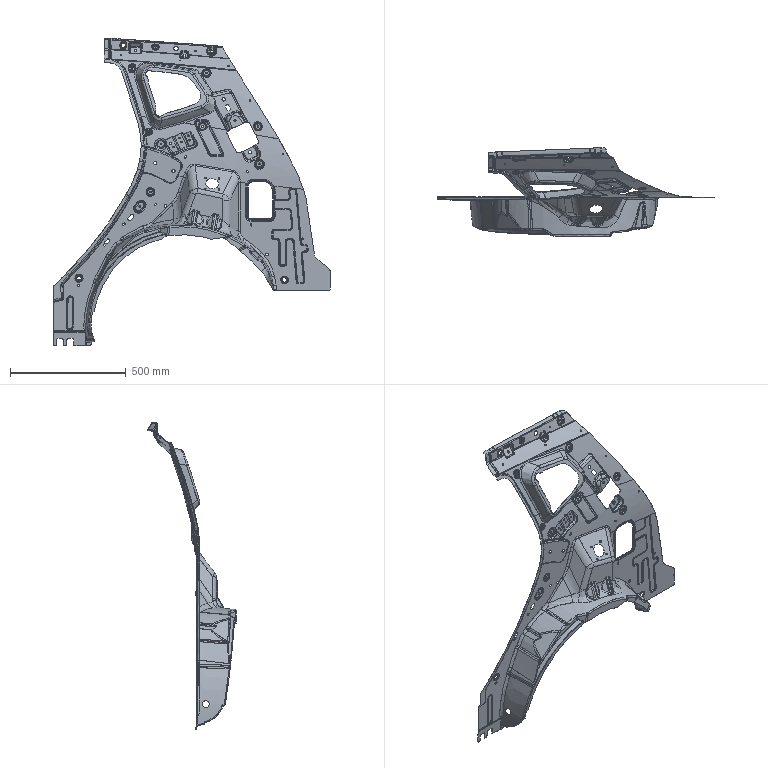Part | STEP file | FNA5401811 | 1 solid | 2173 faces | box 1194 x 381.776 x 1328 mm | volume 682767 mm3 | spline 1709 | cylinder 267 | plane 104 | other 45 | torus 38 | sphere 10 | commonest cylinder face diameters 10 x28 8.4 x24 8 x23 16 x23 14.4 x19 7 x17